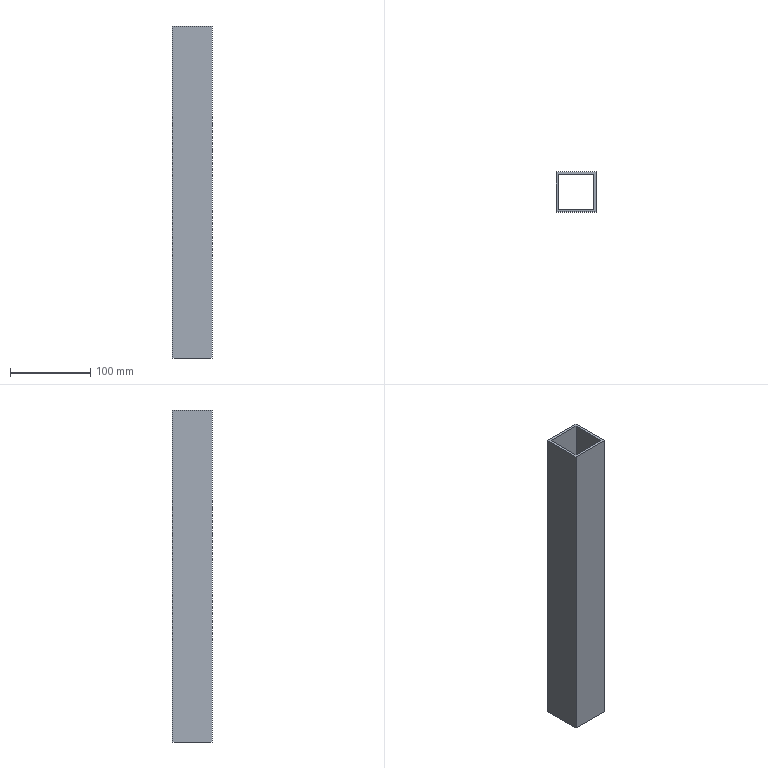Part | SolidWorks | features Extrusion 1 | 1 solid | 10 faces | box 50 x 50 x 415 mm | volume 234060 mm3 | plane 10
STEP:
#1=CARTESIAN_POINT('',(0.,0.,415.));
#2=VERTEX_POINT('',#1);
#3=CARTESIAN_POINT('',(50.,0.,415.));
#4=VERTEX_POINT('',#3);
#5=CARTESIAN_POINT('',(50.,0.,415.));
#6=DIRECTION('',(1.,0.,0.));
#7=VECTOR('',#6,1000.);
#8=LINE('',#5,#7);
#9=EDGE_CURVE('',#2,#4,#8,.T.);
#10=ORIENTED_EDGE('',*,*,#9,.T.);
#11=CARTESIAN_POINT('',(50.,50.,415.));
#12=VERTEX_POINT('',#11);
#13=CARTESIAN_POINT('',(50.,50.,415.));
#14=DIRECTION('',(0.,1.,0.));
#15=VECTOR('',#14,1000.);
#16=LINE('',#13,#15);
#17=EDGE_CURVE('',#4,#12,#16,.T.);
#18=ORIENTED_EDGE('',*,*,#17,.T.);
#19=CARTESIAN_POINT('',(0.,50.,415.));
#20=VERTEX_POINT('',#19);
#21=CARTESIAN_POINT('',(0.,50.,415.));
#22=DIRECTION('',(-1.,0.,0.));
#23=VECTOR('',#22,1000.);
#24=LINE('',#21,#23);
#25=EDGE_CURVE('',#12,#20,#24,.T.);
#26=ORIENTED_EDGE('',*,*,#25,.T.);
#27=CARTESIAN_POINT('',(0.,0.,415.));
#28=DIRECTION('',(0.,-1.,0.));
#29=VECTOR('',#28,1000.);
#30=LINE('',#27,#29);
#31=EDGE_CURVE('',#20,#2,#30,.T.);
#32=ORIENTED_EDGE('',*,*,#31,.T.);
#33=EDGE_LOOP('',(#10,#18,#26,#32));
#34=FACE_OUTER_BOUND('',#33,.T.);
#35=CARTESIAN_POINT('',(3.,3.,415.));
#36=VERTEX_POINT('',#35);
#37=CARTESIAN_POINT('',(47.,3.,415.));
#38=VERTEX_POINT('',#37);
#39=CARTESIAN_POINT('',(47.,3.,415.));
#40=DIRECTION('',(1.,0.,0.));
#41=VECTOR('',#40,1000.);
#42=LINE('',#39,#41);
#43=EDGE_CURVE('',#36,#38,#42,.T.);
#44=ORIENTED_EDGE('',*,*,#43,.F.);
#45=CARTESIAN_POINT('',(3.,47.,415.));
#46=VERTEX_POINT('',#45);
#47=CARTESIAN_POINT('',(3.,3.,415.));
#48=DIRECTION('',(0.,-1.,0.));
#49=VECTOR('',#48,1000.);
#50=LINE('',#47,#49);
#51=EDGE_CURVE('',#46,#36,#50,.T.);
#52=ORIENTED_EDGE('',*,*,#51,.F.);
#53=CARTESIAN_POINT('',(47.,47.,415.));
#54=VERTEX_POINT('',#53);
#55=CARTESIAN_POINT('',(3.,47.,415.));
#56=DIRECTION('',(-1.,0.,0.));
#57=VECTOR('',#56,1000.);
#58=LINE('',#55,#57);
#59=EDGE_CURVE('',#54,#46,#58,.T.);
#60=ORIENTED_EDGE('',*,*,#59,.F.);
#61=CARTESIAN_POINT('',(47.,47.,415.));
#62=DIRECTION('',(0.,1.,0.));
#63=VECTOR('',#62,1000.);
#64=LINE('',#61,#63);
#65=EDGE_CURVE('',#38,#54,#64,.T.);
#66=ORIENTED_EDGE('',*,*,#65,.F.);
#67=EDGE_LOOP('',(#44,#52,#60,#66));
#68=FACE_BOUND('',#67,.T.);
#69=CARTESIAN_POINT('',(0.,0.,415.));
#70=DIRECTION('',(0.,0.,-1.));
#71=DIRECTION('',(-1.,0.,0.));
#72=AXIS2_PLACEMENT_3D('',#69,#70,#71);
#73=PLANE('',#72);
#74=ADVANCED_FACE('',(#34,#68),#73,.F.);
#75=CARTESIAN_POINT('',(0.,0.,0.));
#76=VERTEX_POINT('',#75);
#77=CARTESIAN_POINT('',(50.,0.,0.));
#78=VERTEX_POINT('',#77);
#79=CARTESIAN_POINT('',(50.,0.,0.));
#80=DIRECTION('',(1.,0.,0.));
#81=VECTOR('',#80,1000.);
#82=LINE('',#79,#81);
#83=EDGE_CURVE('',#76,#78,#82,.T.);
#84=ORIENTED_EDGE('',*,*,#83,.F.);
#85=CARTESIAN_POINT('',(0.,50.,0.));
#86=VERTEX_POINT('',#85);
#87=CARTESIAN_POINT('',(0.,0.,0.));
#88=DIRECTION('',(0.,-1.,0.));
#89=VECTOR('',#88,1000.);
#90=LINE('',#87,#89);
#91=EDGE_CURVE('',#86,#76,#90,.T.);
#92=ORIENTED_EDGE('',*,*,#91,.F.);
#93=CARTESIAN_POINT('',(50.,50.,0.));
#94=VERTEX_POINT('',#93);
#95=CARTESIAN_POINT('',(0.,50.,0.));
#96=DIRECTION('',(-1.,0.,0.));
#97=VECTOR('',#96,1000.);
#98=LINE('',#95,#97);
#99=EDGE_CURVE('',#94,#86,#98,.T.);
#100=ORIENTED_EDGE('',*,*,#99,.F.);
#101=CARTESIAN_POINT('',(50.,50.,0.));
#102=DIRECTION('',(0.,1.,0.));
#103=VECTOR('',#102,1000.);
#104=LINE('',#101,#103);
#105=EDGE_CURVE('',#78,#94,#104,.T.);
#106=ORIENTED_EDGE('',*,*,#105,.F.);
#107=EDGE_LOOP('',(#84,#92,#100,#106));
#108=FACE_OUTER_BOUND('',#107,.T.);
#109=CARTESIAN_POINT('',(3.,47.,0.));
#110=VERTEX_POINT('',#109);
#111=CARTESIAN_POINT('',(3.,3.,0.));
#112=VERTEX_POINT('',#111);
#113=CARTESIAN_POINT('',(3.,3.,0.));
#114=DIRECTION('',(0.,-1.,0.));
#115=VECTOR('',#114,1000.);
#116=LINE('',#113,#115);
#117=EDGE_CURVE('',#110,#112,#116,.T.);
#118=ORIENTED_EDGE('',*,*,#117,.T.);
#119=CARTESIAN_POINT('',(47.,3.,0.));
#120=VERTEX_POINT('',#119);
#121=CARTESIAN_POINT('',(47.,3.,0.));
#122=DIRECTION('',(1.,0.,0.));
#123=VECTOR('',#122,1000.);
#124=LINE('',#121,#123);
#125=EDGE_CURVE('',#112,#120,#124,.T.);
#126=ORIENTED_EDGE('',*,*,#125,.T.);
#127=CARTESIAN_POINT('',(47.,47.,0.));
#128=VERTEX_POINT('',#127);
#129=CARTESIAN_POINT('',(47.,47.,0.));
#130=DIRECTION('',(0.,1.,0.));
#131=VECTOR('',#130,1000.);
#132=LINE('',#129,#131);
#133=EDGE_CURVE('',#120,#128,#132,.T.);
#134=ORIENTED_EDGE('',*,*,#133,.T.);
#135=CARTESIAN_POINT('',(3.,47.,0.));
#136=DIRECTION('',(-1.,0.,0.));
#137=VECTOR('',#136,1000.);
#138=LINE('',#135,#137);
#139=EDGE_CURVE('',#128,#110,#138,.T.);
#140=ORIENTED_EDGE('',*,*,#139,.T.);
#141=EDGE_LOOP('',(#118,#126,#134,#140));
#142=FACE_BOUND('',#141,.T.);
#143=CARTESIAN_POINT('',(0.,0.,0.));
#144=DIRECTION('',(0.,0.,-1.));
#145=DIRECTION('',(-1.,0.,0.));
#146=AXIS2_PLACEMENT_3D('',#143,#144,#145);
#147=PLANE('',#146);
#148=ADVANCED_FACE('',(#108,#142),#147,.T.);
#149=ORIENTED_EDGE('',*,*,#83,.T.);
#150=CARTESIAN_POINT('',(50.,0.,415.));
#151=DIRECTION('',(0.,0.,-1.));
#152=VECTOR('',#151,1000.);
#153=LINE('',#150,#152);
#154=EDGE_CURVE('',#4,#78,#153,.T.);
#155=ORIENTED_EDGE('',*,*,#154,.F.);
#156=ORIENTED_EDGE('',*,*,#9,.F.);
#157=CARTESIAN_POINT('',(0.,0.,415.));
#158=DIRECTION('',(0.,0.,-1.));
#159=VECTOR('',#158,1000.);
#160=LINE('',#157,#159);
#161=EDGE_CURVE('',#2,#76,#160,.T.);
#162=ORIENTED_EDGE('',*,*,#161,.T.);
#163=EDGE_LOOP('',(#149,#155,#156,#162));
#164=FACE_OUTER_BOUND('',#163,.T.);
#165=CARTESIAN_POINT('',(50.,0.,415.));
#166=DIRECTION('',(0.,1.,0.));
#167=DIRECTION('',(0.,0.,1.));
#168=AXIS2_PLACEMENT_3D('',#165,#166,#167);
#169=PLANE('',#168);
#170=ADVANCED_FACE('',(#164),#169,.F.);
#171=ORIENTED_EDGE('',*,*,#105,.T.);
#172=CARTESIAN_POINT('',(50.,50.,415.));
#173=DIRECTION('',(0.,0.,-1.));
#174=VECTOR('',#173,1000.);
#175=LINE('',#172,#174);
#176=EDGE_CURVE('',#12,#94,#175,.T.);
#177=ORIENTED_EDGE('',*,*,#176,.F.);
#178=ORIENTED_EDGE('',*,*,#17,.F.);
#179=ORIENTED_EDGE('',*,*,#154,.T.);
#180=EDGE_LOOP('',(#171,#177,#178,#179));
#181=FACE_OUTER_BOUND('',#180,.T.);
#182=CARTESIAN_POINT('',(50.,50.,415.));
#183=DIRECTION('',(-1.,0.,0.));
#184=DIRECTION('',(0.,0.,1.));
#185=AXIS2_PLACEMENT_3D('',#182,#183,#184);
#186=PLANE('',#185);
#187=ADVANCED_FACE('',(#181),#186,.F.);
#188=ORIENTED_EDGE('',*,*,#99,.T.);
#189=CARTESIAN_POINT('',(0.,50.,415.));
#190=DIRECTION('',(0.,0.,-1.));
#191=VECTOR('',#190,1000.);
#192=LINE('',#189,#191);
#193=EDGE_CURVE('',#20,#86,#192,.T.);
#194=ORIENTED_EDGE('',*,*,#193,.F.);
#195=ORIENTED_EDGE('',*,*,#25,.F.);
#196=ORIENTED_EDGE('',*,*,#176,.T.);
#197=EDGE_LOOP('',(#188,#194,#195,#196));
#198=FACE_OUTER_BOUND('',#197,.T.);
#199=CARTESIAN_POINT('',(0.,50.,415.));
#200=DIRECTION('',(0.,-1.,0.));
#201=DIRECTION('',(0.,0.,-1.));
#202=AXIS2_PLACEMENT_3D('',#199,#200,#201);
#203=PLANE('',#202);
#204=ADVANCED_FACE('',(#198),#203,.F.);
#205=ORIENTED_EDGE('',*,*,#91,.T.);
#206=ORIENTED_EDGE('',*,*,#161,.F.);
#207=ORIENTED_EDGE('',*,*,#31,.F.);
#208=ORIENTED_EDGE('',*,*,#193,.T.);
#209=EDGE_LOOP('',(#205,#206,#207,#208));
#210=FACE_OUTER_BOUND('',#209,.T.);
#211=CARTESIAN_POINT('',(0.,0.,415.));
#212=DIRECTION('',(1.,0.,0.));
#213=DIRECTION('',(0.,0.,-1.));
#214=AXIS2_PLACEMENT_3D('',#211,#212,#213);
#215=PLANE('',#214);
#216=ADVANCED_FACE('',(#210),#215,.F.);
#217=ORIENTED_EDGE('',*,*,#125,.F.);
#218=CARTESIAN_POINT('',(3.,3.,415.));
#219=DIRECTION('',(0.,0.,-1.));
#220=VECTOR('',#219,1000.);
#221=LINE('',#218,#220);
#222=EDGE_CURVE('',#36,#112,#221,.T.);
#223=ORIENTED_EDGE('',*,*,#222,.F.);
#224=ORIENTED_EDGE('',*,*,#43,.T.);
#225=CARTESIAN_POINT('',(47.,3.,415.));
#226=DIRECTION('',(0.,0.,-1.));
#227=VECTOR('',#226,1000.);
#228=LINE('',#225,#227);
#229=EDGE_CURVE('',#38,#120,#228,.T.);
#230=ORIENTED_EDGE('',*,*,#229,.T.);
#231=EDGE_LOOP('',(#217,#223,#224,#230));
#232=FACE_OUTER_BOUND('',#231,.T.);
#233=CARTESIAN_POINT('',(47.,3.,415.));
#234=DIRECTION('',(0.,1.,0.));
#235=DIRECTION('',(0.,0.,1.));
#236=AXIS2_PLACEMENT_3D('',#233,#234,#235);
#237=PLANE('',#236);
#238=ADVANCED_FACE('',(#232),#237,.T.);
#239=ORIENTED_EDGE('',*,*,#133,.F.);
#240=ORIENTED_EDGE('',*,*,#229,.F.);
#241=ORIENTED_EDGE('',*,*,#65,.T.);
#242=CARTESIAN_POINT('',(47.,47.,415.));
#243=DIRECTION('',(0.,0.,-1.));
#244=VECTOR('',#243,1000.);
#245=LINE('',#242,#244);
#246=EDGE_CURVE('',#54,#128,#245,.T.);
#247=ORIENTED_EDGE('',*,*,#246,.T.);
#248=EDGE_LOOP('',(#239,#240,#241,#247));
#249=FACE_OUTER_BOUND('',#248,.T.);
#250=CARTESIAN_POINT('',(47.,47.,415.));
#251=DIRECTION('',(-1.,0.,0.));
#252=DIRECTION('',(0.,0.,1.));
#253=AXIS2_PLACEMENT_3D('',#250,#251,#252);
#254=PLANE('',#253);
#255=ADVANCED_FACE('',(#249),#254,.T.);
#256=ORIENTED_EDGE('',*,*,#139,.F.);
#257=ORIENTED_EDGE('',*,*,#246,.F.);
#258=ORIENTED_EDGE('',*,*,#59,.T.);
#259=CARTESIAN_POINT('',(3.,47.,415.));
#260=DIRECTION('',(0.,0.,-1.));
#261=VECTOR('',#260,1000.);
#262=LINE('',#259,#261);
#263=EDGE_CURVE('',#46,#110,#262,.T.);
#264=ORIENTED_EDGE('',*,*,#263,.T.);
#265=EDGE_LOOP('',(#256,#257,#258,#264));
#266=FACE_OUTER_BOUND('',#265,.T.);
#267=CARTESIAN_POINT('',(3.,47.,415.));
#268=DIRECTION('',(0.,-1.,0.));
#269=DIRECTION('',(0.,0.,-1.));
#270=AXIS2_PLACEMENT_3D('',#267,#268,#269);
#271=PLANE('',#270);
#272=ADVANCED_FACE('',(#266),#271,.T.);
#273=ORIENTED_EDGE('',*,*,#117,.F.);
#274=ORIENTED_EDGE('',*,*,#263,.F.);
#275=ORIENTED_EDGE('',*,*,#51,.T.);
#276=ORIENTED_EDGE('',*,*,#222,.T.);
#277=EDGE_LOOP('',(#273,#274,#275,#276));
#278=FACE_OUTER_BOUND('',#277,.T.);
#279=CARTESIAN_POINT('',(3.,3.,415.));
#280=DIRECTION('',(1.,0.,0.));
#281=DIRECTION('',(0.,0.,-1.));
#282=AXIS2_PLACEMENT_3D('',#279,#280,#281);
#283=PLANE('',#282);
#284=ADVANCED_FACE('',(#278),#283,.T.);
#285=CLOSED_SHELL('',(#74,#148,#170,#187,#204,#216,#238,#255,#272,#284));
#286=MANIFOLD_SOLID_BREP('',#285);
#287=CARTESIAN_POINT('',(0.,0.,0.));
#288=DIRECTION('',(0.,0.,1.));
#289=DIRECTION('',(1.,0.,0.));
#290=AXIS2_PLACEMENT_3D('',#287,#288,#289);
#291=(LENGTH_UNIT()NAMED_UNIT(*)SI_UNIT(.MILLI.,.METRE.));
#292=UNCERTAINTY_MEASURE_WITH_UNIT(LENGTH_MEASURE(0.00001),#291,'','');
#293=(NAMED_UNIT(*)PLANE_ANGLE_UNIT()SI_UNIT($,.RADIAN.));
#294=(NAMED_UNIT(*)SI_UNIT($,.STERADIAN.)SOLID_ANGLE_UNIT());
#295=(GEOMETRIC_REPRESENTATION_CONTEXT(3)GLOBAL_UNCERTAINTY_ASSIGNED_CONTEXT((#292))GLOBAL_UNIT_ASSIGNED_CONTEXT((#291,#293,#294))REPRESENTATION_CONTEXT('',''));
#296=ADVANCED_BREP_SHAPE_REPRESENTATION('',(#286,#290),#295);